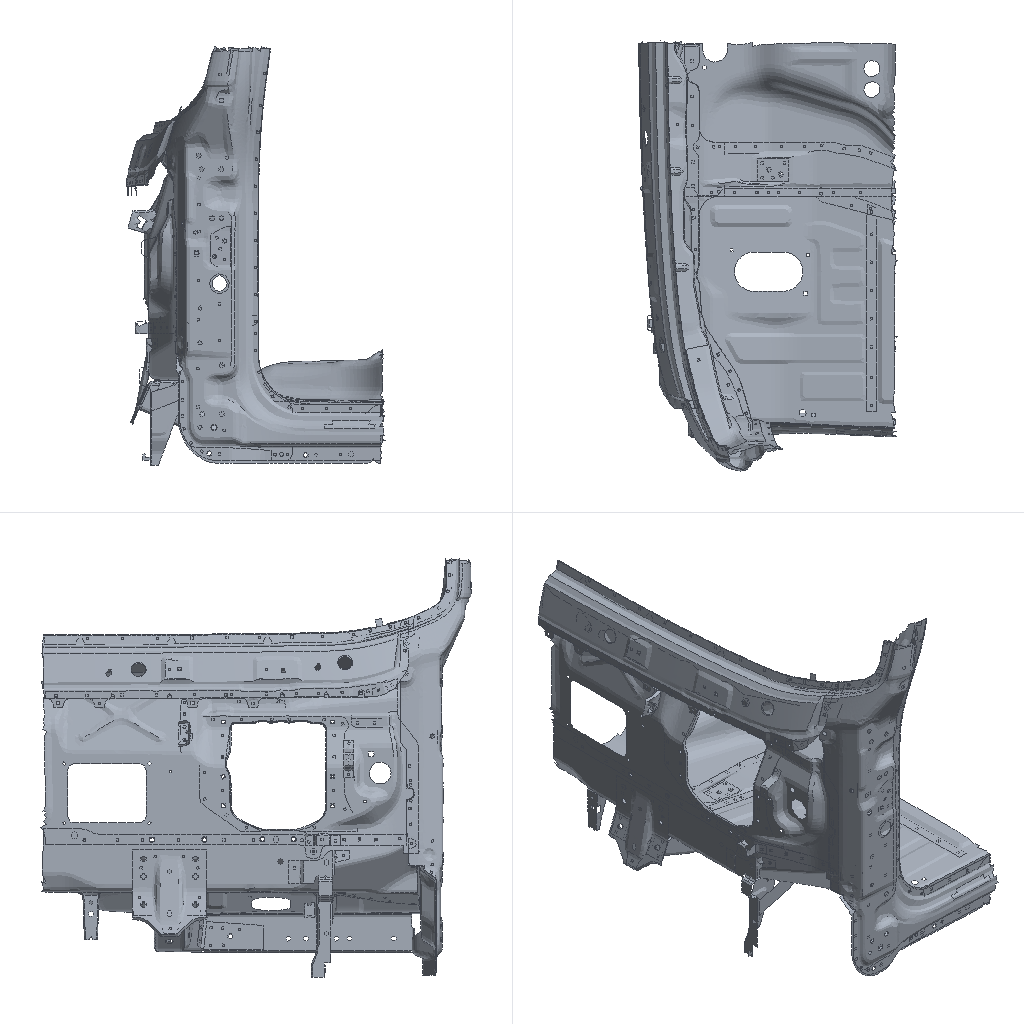Simulation study | nastran
Set-up summary:
category,name,step,type,value,unit,region
solver,nx_nastran
units,not stated in the deck,,not stated
analysis,deck,,static,static
analysis,solution,,SOL,101
load_step,SUBCASE 1,1,SUBCASE,SPC=7 LOAD=1
load_step,SUBCASE 2,2,SUBCASE,SPC=7 LOAD=2
load_step,SUBCASE 3,3,SUBCASE,SPC=7 LOAD=3
load_step,SUBCASE 4,4,SUBCASE,SPC=7 LOAD=4
load_step,SUBCASE 5,5,SUBCASE,SPC=7 LOAD=5
load_step,SUBCASE 6,6,SUBCASE,SPC=7 LOAD=6
load_step,requested,,,6
mesh,nodes,,,41795
mesh,elements,,,37377
element_type,CHEXA,,unverified,346
element_type,CQUAD4,,shell,34683
element_type,CTRIA3,,shell,2694
load,load commands in deck,,count,6
bc,support commands in deck,,count,1066
check,setup vs results,,match,"every grid point's frame and coordinates and every element id; grid points of CHEXA, CQUAD4, CTRIA3 elements"
Nastran input file, long lists of numbers shortened:
$$------------------------------------------------------------------------------$
$$                                                                              $
$$ NASTRAN Input Deck Generated by HyperMesh Version  : 9.0b121                 $
$$ Generated using HyperMesh-Nastran Template Version : 9.0b121
$$                                                                              $
$$   Template:  general                                                         $
$$                                                                              $
$$------------------------------------------------------------------------------$
$$------------------------------------------------------------------------------$
$$                      Executive Control Cards                                 $
$$------------------------------------------------------------------------------$
SOL 101
CEND
$$------------------------------------------------------------------------------$
$$                      Case Control Cards                                      $
$$------------------------------------------------------------------------------$
  DISPLACEMENT(PLOT) = ALL
  STRESS(PLOT) = ALL
$
$HMNAME LOADSTEP               1"Lx"
SUBCASE       1
  LABEL=  Lx
  SPC =        7
  LOAD =        1
$
$HMNAME LOADSTEP               2"Ly"
SUBCASE       2
  LABEL=  Ly
  SPC =        7
  LOAD =        2
$
$HMNAME LOADSTEP               3"Lz"
SUBCASE       3
  LABEL=  Lz
  SPC =        7
  LOAD =        3
$
$HMNAME LOADSTEP               4"Rx"
SUBCASE       4
  LABEL=  Rx
  SPC =        7
  LOAD =        4
$
$HMNAME LOADSTEP               5"Ry"
SUBCASE       5
  LABEL=  Ry
  SPC =        7
  LOAD =        5
$
$HMNAME LOADSTEP               6"Rz"
SUBCASE       6
  LABEL=  Rz
  SPC =        7
  LOAD =        6
$$------------------------------------------------------------------------------$
$$                      Bulk Data Cards                                         $
$$------------------------------------------------------------------------------$
BEGIN BULK
PARAM,BAILOUT,-1
PARAM,POST,-1
$$
$$  GRID Data
$$
GRID         150        -903.017-1033.041012.706
GRID         536        -985.883-1013.11735.4542
$ (41793 more lines like these left out)
$$
$$  SPOINT Data
$$
$$
$$------------------------------------------------------------------------------$
$$             Group Definitions                                                $
$$------------------------------------------------------------------------------$
$
$ RBE2 Elements - Single dependent node
$
RBE2      346590 3663307  123456 3657894
RBE2      346592 3663309  123456 3657892
$ (9 more lines like these left out)
$
$HMMOVE 57005014
$         346590  346592THRU      346597  346600THRU      346603
$
$$
$$ RBE2 Elements - Multiple dependent nodes
$$
RBE2      346588 3663313  123456 3658184 3658185
RBE2      346589 3663312  123456 3657889 3658186
$ (78 more lines like these left out)
$
$HMMOVE 57005014
$         346588THRU      346589  346591  346598THRU      346599  346625THRU
$         346630  346920 1034945THRU     1034946
$
$
$  RBE3 Elements
$
RBE3      326805         3755900  1234560.023859     123 37185220.266194+
+            123 37185270.651549     123 37185210.058398     123 3718516
RBE3      326806         3755901  1234560.041766     123 37185160.685126+
+            123 37185210.257415     123 37185150.015692     123 3718509
$ (5532 more lines like these left out)
$
$HMMOVE 57005012
$         326805THRU      326808  326810THRU      326817  326819THRU      326826
$         326828THRU      326835  326837THRU      326844  326846THRU      326853
$ (139 more lines like these left out)
CTRIA3    143987       2   55842   55843   55841
CTRIA3    144058       2   55842   55841   55996
$ (2692 more lines like these left out)
$
$HMMOVE       16
$         143987  144058  170026  170031  170036THRU      170037  170041  170048
$         170053  170057THRU      170058  189522  189524  198834THRU      198835
$ (336 more lines like these left out)
CQUAD4    170025       2   86431   86432   86426   86427
CQUAD4    170027       2   86442   86467   86451   86441
$ (34681 more lines like these left out)
$
$HMMOVE       16
$         170025  170027THRU      170030  170032THRU      170035  170038THRU
$         170040  170042THRU      170047  170049THRU      170052  170054THRU
$ (900 more lines like these left out)
CHEXA     326809      10 3755900 3755901 3755902 3755903 3755904 3755905+
+        3755906 3755907
CHEXA     326818      10 3755909 3755912 3755911 3755910 3755913 3755916+
+        3755915 3755914
$ (688 more lines like these left out)
$
$HMMOVE 57005011
$         326809  326818  326827  326836  326845  326854  326881  326890  326899
$         326908  326917  326926  326935  326944  326953  326962  326971  326980
$ (164 more lines like these left out)
PSHELL         1       10.8            1               1
$
$HMNAME PROP                   2"120" 4
$HWCOLOR PROP                  2       3
PSHELL         2       11.2            1               1
$
$HMNAME PROP                   3"180" 4
$HWCOLOR PROP                  3       3
PSHELL         3       11.8            1               1
$
$HMNAME PROP                   4"100" 4
$HWCOLOR PROP                  4       3
PSHELL         4       11.0            1               1
$
$HMNAME PROP                   5"150" 4
$HWCOLOR PROP                  5       3
PSHELL         5       11.5            1               1
$
$HMNAME PROP                   6"250" 4
$HWCOLOR PROP                  6       3
PSHELL         6       12.5            1               1
$
$HMNAME PROP                   7"200" 4
$HWCOLOR PROP                  7       3
PSHELL         7       12.0            1               1
$$
$$  PSOLID Data
$
$HMNAME PROP                  10"spot" 5
$HWCOLOR PROP                 10       3
PSOLID        10       1
$$
$$------------------------------------------------------------------------------$
$$                      Material Definition Cards                               $
$$------------------------------------------------------------------------------$
$$--------------------------------------------------------------
$$ HYPERMESH TAGS
$$--------------------------------------------------------------
$$BEGIN TAGS
$$END TAGS
$$
$$  MAT1 Data
$
$HMNAME MAT                    1"steel" "MAT1"
$HWCOLOR MAT                   1       3
MAT1           1210000.0        0.3     1.60E-08
$$
$$
$$
$$------------------------------------------------------------------------------$
$ (52 more lines like these left out)
SPC            7   95153  1234560.0
SPC            7   95172  1234560.0
SPC            7   95173  1234560.0
SPC            7   95177  1234560.0
$ (1062 more lines like these left out)
$$
$$  FORCE Data
$$
FORCE          184122634       01.0     1000.0  0.0     0.0
FORCE          284122634       01.0     0.0     1000.0  0.0
FORCE          384122634       01.0     0.0     0.0     1000.0
FORCE          484122635       01.0     1000.0  0.0     0.0
FORCE          584122635       01.0     0.0     1000.0  0.0
FORCE          684122635       01.0     0.0     0.0     1000.0
$HMASSEM       1       3 REAR_FLOOR
$HMASSEM_IDS    5100301051001110510052115100931051004510510042105100481151004311
$HMASSEM_IDS    5100461051005410510070105100721051005610510056115100431051005010
$HMASSEM_IDS    5100341051009711
$HMASSEM      28       4 5300010
$HMASSEM_IDS          16      18      20      21      22      24      25      26
$HMASSEM 5400100       7 sidebody_L
$HMASSEM_IDS    5400101054003020540011105400112054003010
$
ENDDATA
Results summary:
result,analysis,,,static
result,last_loadstep,,,6
result,primary field,,,displacements
result,max displacement,,,0.3157,model units